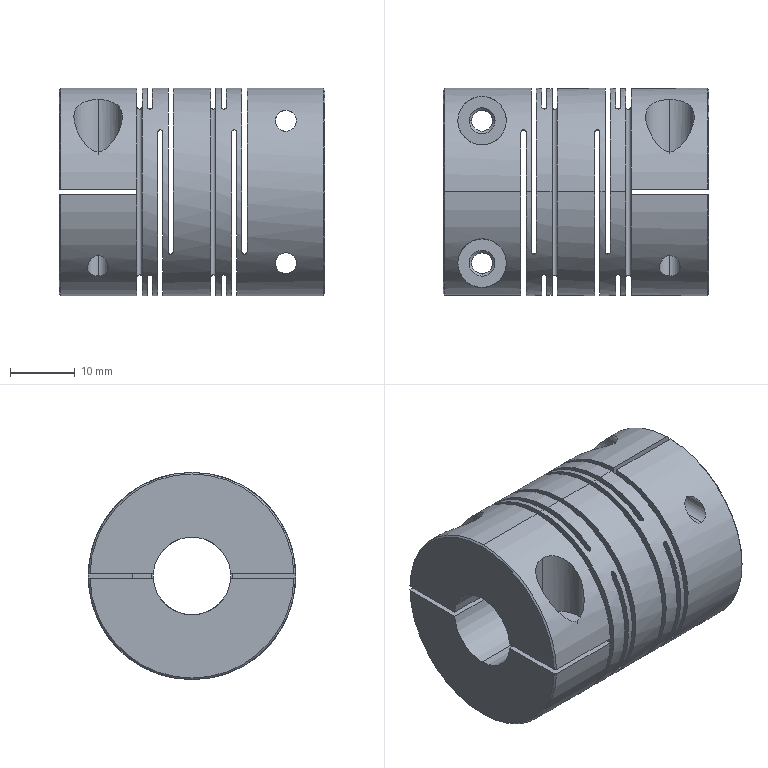Part | STEP file | 0230_Z_007_CPLCN32-12-12_1 | 1 solid | 109 faces | box 41 x 32 x 32 mm | volume 22249 mm3 | cylinder 60 | plane 36 | cone 13 | commonest cylinder face diameters 12.5 x14 0.8 x10 3.242 x8 4 x8 7.5 x8 32 x7